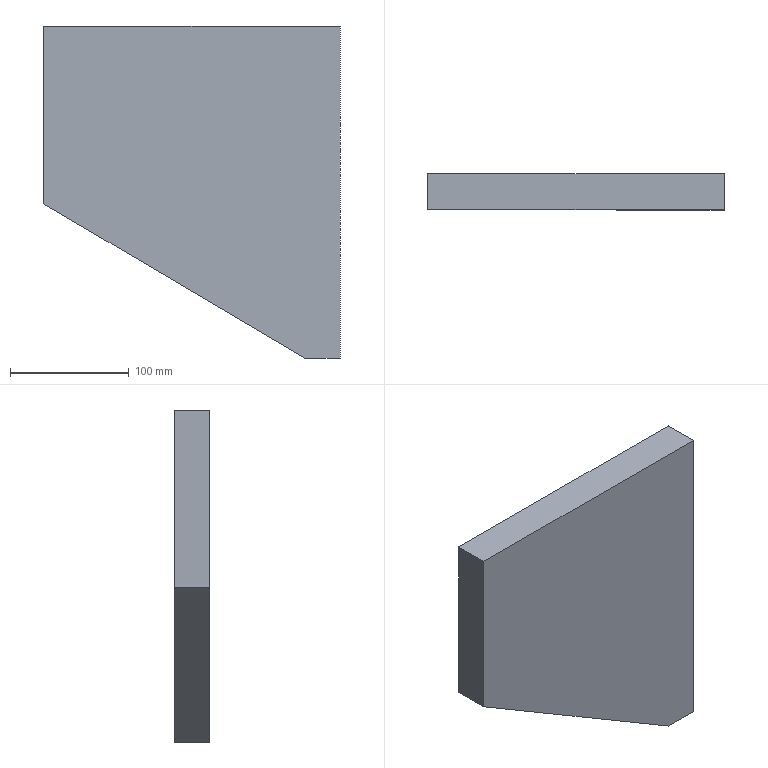Part | SolidWorks | features Extrusion 1 | 1 solid | 7 faces | box 250 x 30 x 280 mm | volume 1671000 mm3 | plane 7
STEP:
#1=CARTESIAN_POINT('',(162.791,0.,97.674));
#2=VERTEX_POINT('',#1);
#3=CARTESIAN_POINT('',(162.791,0.,-182.326));
#4=VERTEX_POINT('',#3);
#5=CARTESIAN_POINT('',(162.791,0.,97.674));
#6=DIRECTION('',(0.,0.,-1.));
#7=VECTOR('',#6,1000.);
#8=LINE('',#5,#7);
#9=EDGE_CURVE('',#2,#4,#8,.T.);
#10=ORIENTED_EDGE('',*,*,#9,.T.);
#11=CARTESIAN_POINT('',(162.791,30.,-182.326));
#12=VERTEX_POINT('',#11);
#13=CARTESIAN_POINT('',(162.791,30.,-182.326));
#14=DIRECTION('',(0.,-1.,0.));
#15=VECTOR('',#14,1000.);
#16=LINE('',#13,#15);
#17=EDGE_CURVE('',#12,#4,#16,.T.);
#18=ORIENTED_EDGE('',*,*,#17,.F.);
#19=CARTESIAN_POINT('',(162.791,30.,97.674));
#20=VERTEX_POINT('',#19);
#21=CARTESIAN_POINT('',(162.791,30.,97.674));
#22=DIRECTION('',(0.,0.,-1.));
#23=VECTOR('',#22,1000.);
#24=LINE('',#21,#23);
#25=EDGE_CURVE('',#20,#12,#24,.T.);
#26=ORIENTED_EDGE('',*,*,#25,.F.);
#27=CARTESIAN_POINT('',(162.791,30.,97.674));
#28=DIRECTION('',(0.,-1.,0.));
#29=VECTOR('',#28,1000.);
#30=LINE('',#27,#29);
#31=EDGE_CURVE('',#20,#2,#30,.T.);
#32=ORIENTED_EDGE('',*,*,#31,.T.);
#33=EDGE_LOOP('',(#10,#18,#26,#32));
#34=FACE_OUTER_BOUND('',#33,.T.);
#35=CARTESIAN_POINT('',(162.791,30.,97.674));
#36=DIRECTION('',(-1.,0.,0.));
#37=DIRECTION('',(0.,0.,1.));
#38=AXIS2_PLACEMENT_3D('',#35,#36,#37);
#39=PLANE('',#38);
#40=ADVANCED_FACE('',(#34),#39,.F.);
#41=CARTESIAN_POINT('',(132.791,0.,-182.326));
#42=VERTEX_POINT('',#41);
#43=CARTESIAN_POINT('',(162.791,0.,-182.326));
#44=DIRECTION('',(-1.,0.,0.));
#45=VECTOR('',#44,1000.);
#46=LINE('',#43,#45);
#47=EDGE_CURVE('',#4,#42,#46,.T.);
#48=ORIENTED_EDGE('',*,*,#47,.T.);
#49=CARTESIAN_POINT('',(132.791,30.,-182.326));
#50=VERTEX_POINT('',#49);
#51=CARTESIAN_POINT('',(132.791,30.,-182.326));
#52=DIRECTION('',(0.,-1.,0.));
#53=VECTOR('',#52,1000.);
#54=LINE('',#51,#53);
#55=EDGE_CURVE('',#50,#42,#54,.T.);
#56=ORIENTED_EDGE('',*,*,#55,.F.);
#57=CARTESIAN_POINT('',(162.791,30.,-182.326));
#58=DIRECTION('',(-1.,0.,0.));
#59=VECTOR('',#58,1000.);
#60=LINE('',#57,#59);
#61=EDGE_CURVE('',#12,#50,#60,.T.);
#62=ORIENTED_EDGE('',*,*,#61,.F.);
#63=ORIENTED_EDGE('',*,*,#17,.T.);
#64=EDGE_LOOP('',(#48,#56,#62,#63));
#65=FACE_OUTER_BOUND('',#64,.T.);
#66=CARTESIAN_POINT('',(162.791,30.,-182.326));
#67=DIRECTION('',(0.,0.,1.));
#68=DIRECTION('',(1.,0.,0.));
#69=AXIS2_PLACEMENT_3D('',#66,#67,#68);
#70=PLANE('',#69);
#71=ADVANCED_FACE('',(#65),#70,.F.);
#72=CARTESIAN_POINT('',(-87.209,0.,-52.326));
#73=VERTEX_POINT('',#72);
#74=CARTESIAN_POINT('',(132.791,0.,-182.326));
#75=DIRECTION('',(-0.8609,0.,0.5087));
#76=VECTOR('',#75,1000.);
#77=LINE('',#74,#76);
#78=EDGE_CURVE('',#42,#73,#77,.T.);
#79=ORIENTED_EDGE('',*,*,#78,.T.);
#80=CARTESIAN_POINT('',(-87.209,30.,-52.326));
#81=VERTEX_POINT('',#80);
#82=CARTESIAN_POINT('',(-87.209,30.,-52.326));
#83=DIRECTION('',(0.,-1.,0.));
#84=VECTOR('',#83,1000.);
#85=LINE('',#82,#84);
#86=EDGE_CURVE('',#81,#73,#85,.T.);
#87=ORIENTED_EDGE('',*,*,#86,.F.);
#88=CARTESIAN_POINT('',(132.791,30.,-182.326));
#89=DIRECTION('',(-0.8609,0.,0.5087));
#90=VECTOR('',#89,1000.);
#91=LINE('',#88,#90);
#92=EDGE_CURVE('',#50,#81,#91,.T.);
#93=ORIENTED_EDGE('',*,*,#92,.F.);
#94=ORIENTED_EDGE('',*,*,#55,.T.);
#95=EDGE_LOOP('',(#79,#87,#93,#94));
#96=FACE_OUTER_BOUND('',#95,.T.);
#97=CARTESIAN_POINT('',(132.791,30.,-182.326));
#98=DIRECTION('',(0.5087,0.,0.8609));
#99=DIRECTION('',(0.8609,0.,-0.5087));
#100=AXIS2_PLACEMENT_3D('',#97,#98,#99);
#101=PLANE('',#100);
#102=ADVANCED_FACE('',(#96),#101,.F.);
#103=CARTESIAN_POINT('',(-87.209,0.,97.674));
#104=VERTEX_POINT('',#103);
#105=CARTESIAN_POINT('',(-87.209,0.,97.674));
#106=DIRECTION('',(0.,0.,1.));
#107=VECTOR('',#106,1000.);
#108=LINE('',#105,#107);
#109=EDGE_CURVE('',#73,#104,#108,.T.);
#110=ORIENTED_EDGE('',*,*,#109,.T.);
#111=CARTESIAN_POINT('',(-87.209,30.,97.674));
#112=VERTEX_POINT('',#111);
#113=CARTESIAN_POINT('',(-87.209,30.,97.674));
#114=DIRECTION('',(0.,-1.,0.));
#115=VECTOR('',#114,1000.);
#116=LINE('',#113,#115);
#117=EDGE_CURVE('',#112,#104,#116,.T.);
#118=ORIENTED_EDGE('',*,*,#117,.F.);
#119=CARTESIAN_POINT('',(-87.209,30.,97.674));
#120=DIRECTION('',(0.,0.,1.));
#121=VECTOR('',#120,1000.);
#122=LINE('',#119,#121);
#123=EDGE_CURVE('',#81,#112,#122,.T.);
#124=ORIENTED_EDGE('',*,*,#123,.F.);
#125=ORIENTED_EDGE('',*,*,#86,.T.);
#126=EDGE_LOOP('',(#110,#118,#124,#125));
#127=FACE_OUTER_BOUND('',#126,.T.);
#128=CARTESIAN_POINT('',(-87.209,30.,97.674));
#129=DIRECTION('',(1.,0.,0.));
#130=DIRECTION('',(0.,0.,-1.));
#131=AXIS2_PLACEMENT_3D('',#128,#129,#130);
#132=PLANE('',#131);
#133=ADVANCED_FACE('',(#127),#132,.F.);
#134=CARTESIAN_POINT('',(-87.209,0.,97.674));
#135=DIRECTION('',(1.,0.,0.));
#136=VECTOR('',#135,1000.);
#137=LINE('',#134,#136);
#138=EDGE_CURVE('',#104,#2,#137,.T.);
#139=ORIENTED_EDGE('',*,*,#138,.T.);
#140=ORIENTED_EDGE('',*,*,#31,.F.);
#141=CARTESIAN_POINT('',(-87.209,30.,97.674));
#142=DIRECTION('',(1.,0.,0.));
#143=VECTOR('',#142,1000.);
#144=LINE('',#141,#143);
#145=EDGE_CURVE('',#112,#20,#144,.T.);
#146=ORIENTED_EDGE('',*,*,#145,.F.);
#147=ORIENTED_EDGE('',*,*,#117,.T.);
#148=EDGE_LOOP('',(#139,#140,#146,#147));
#149=FACE_OUTER_BOUND('',#148,.T.);
#150=CARTESIAN_POINT('',(-87.209,30.,97.674));
#151=DIRECTION('',(0.,0.,-1.));
#152=DIRECTION('',(-1.,0.,0.));
#153=AXIS2_PLACEMENT_3D('',#150,#151,#152);
#154=PLANE('',#153);
#155=ADVANCED_FACE('',(#149),#154,.F.);
#156=ORIENTED_EDGE('',*,*,#25,.T.);
#157=ORIENTED_EDGE('',*,*,#61,.T.);
#158=ORIENTED_EDGE('',*,*,#92,.T.);
#159=ORIENTED_EDGE('',*,*,#123,.T.);
#160=ORIENTED_EDGE('',*,*,#145,.T.);
#161=EDGE_LOOP('',(#156,#157,#158,#159,#160));
#162=FACE_OUTER_BOUND('',#161,.T.);
#163=CARTESIAN_POINT('',(0.,30.,0.));
#164=DIRECTION('',(0.,1.,0.));
#165=DIRECTION('',(0.,0.,1.));
#166=AXIS2_PLACEMENT_3D('',#163,#164,#165);
#167=PLANE('',#166);
#168=ADVANCED_FACE('',(#162),#167,.T.);
#169=ORIENTED_EDGE('',*,*,#9,.F.);
#170=ORIENTED_EDGE('',*,*,#138,.F.);
#171=ORIENTED_EDGE('',*,*,#109,.F.);
#172=ORIENTED_EDGE('',*,*,#78,.F.);
#173=ORIENTED_EDGE('',*,*,#47,.F.);
#174=EDGE_LOOP('',(#169,#170,#171,#172,#173));
#175=FACE_OUTER_BOUND('',#174,.T.);
#176=CARTESIAN_POINT('',(0.,0.,0.));
#177=DIRECTION('',(0.,1.,0.));
#178=DIRECTION('',(0.,0.,1.));
#179=AXIS2_PLACEMENT_3D('',#176,#177,#178);
#180=PLANE('',#179);
#181=ADVANCED_FACE('',(#175),#180,.F.);
#182=CLOSED_SHELL('',(#40,#71,#102,#133,#155,#168,#181));
#183=MANIFOLD_SOLID_BREP('',#182);
#184=CARTESIAN_POINT('',(0.,0.,0.));
#185=DIRECTION('',(0.,0.,1.));
#186=DIRECTION('',(1.,0.,0.));
#187=AXIS2_PLACEMENT_3D('',#184,#185,#186);
#188=(LENGTH_UNIT()NAMED_UNIT(*)SI_UNIT(.MILLI.,.METRE.));
#189=UNCERTAINTY_MEASURE_WITH_UNIT(LENGTH_MEASURE(0.00001),#188,'','');
#190=(NAMED_UNIT(*)PLANE_ANGLE_UNIT()SI_UNIT($,.RADIAN.));
#191=(NAMED_UNIT(*)SI_UNIT($,.STERADIAN.)SOLID_ANGLE_UNIT());
#192=(GEOMETRIC_REPRESENTATION_CONTEXT(3)GLOBAL_UNCERTAINTY_ASSIGNED_CONTEXT((#189))GLOBAL_UNIT_ASSIGNED_CONTEXT((#188,#190,#191))REPRESENTATION_CONTEXT('',''));
#193=ADVANCED_BREP_SHAPE_REPRESENTATION('',(#183,#187),#192);